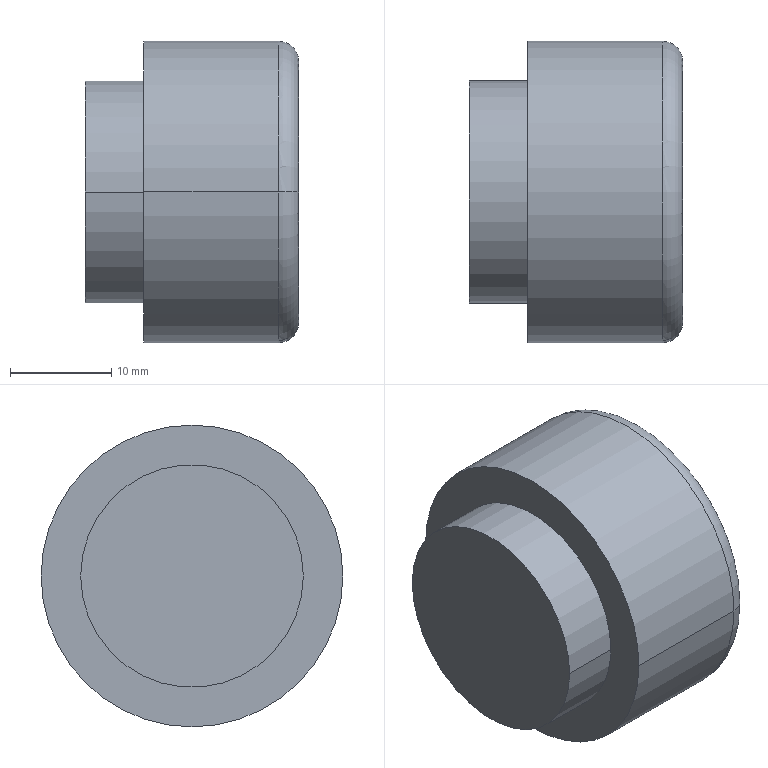Part | STEP file | 7-4-Part3-619-724 | 1 solid | 9 faces | box 21.06 x 29.813 x 29.813 mm | volume 12789 mm3 | cylinder 4 | plane 3 | torus 2 | commonest cylinder face diameters 22 x2 29.813 x2
STEP:
#1=CARTESIAN_POINT('',(0.,0.,0.));
#2=DIRECTION('',(0.,0.,1.));
#3=DIRECTION('',(1.,0.,0.));
#4=AXIS2_PLACEMENT_3D('',#1,#2,#3);
#5=CARTESIAN_POINT('',(19.06,-25.906,0.));
#6=VERTEX_POINT('',#5);
#7=CARTESIAN_POINT('',(19.06,3.906,0.));
#8=VERTEX_POINT('',#7);
#9=CARTESIAN_POINT('',(19.06,-11.,0.));
#10=DIRECTION('',(-1.,0.,0.));
#11=DIRECTION('',(0.,1.,0.));
#12=AXIS2_PLACEMENT_3D('',#9,#10,#11);
#13=CIRCLE('',#12,14.906);
#14=CARTESIAN_POINT('',(19.06,-11.,0.));
#15=DIRECTION('',(1.,0.,0.));
#16=DIRECTION('',(0.,1.,0.));
#17=AXIS2_PLACEMENT_3D('',#14,#15,#16);
#18=TOROIDAL_SURFACE('',#17,12.906,2.);
#19=CARTESIAN_POINT('',(3.142,0.));
#20=CARTESIAN_POINT('',(3.094,0.));
#21=CARTESIAN_POINT('',(2.999,0.));
#22=CARTESIAN_POINT('',(2.856,0.));
#23=CARTESIAN_POINT('',(2.713,0.));
#24=CARTESIAN_POINT('',(2.57,0.));
#25=CARTESIAN_POINT('',(2.428,0.));
#26=CARTESIAN_POINT('',(2.285,0.));
#27=CARTESIAN_POINT('',(2.142,0.));
#28=CARTESIAN_POINT('',(1.999,0.));
#29=CARTESIAN_POINT('',(1.856,0.));
#30=CARTESIAN_POINT('',(1.714,0.));
#31=CARTESIAN_POINT('',(1.571,0.));
#32=CARTESIAN_POINT('',(1.428,0.));
#33=CARTESIAN_POINT('',(1.285,0.));
#34=CARTESIAN_POINT('',(1.142,0.));
#35=CARTESIAN_POINT('',(0.9996,0.));
#36=CARTESIAN_POINT('',(0.8568,0.));
#37=CARTESIAN_POINT('',(0.714,0.));
#38=CARTESIAN_POINT('',(0.5712,0.));
#39=CARTESIAN_POINT('',(0.4284,0.));
#40=CARTESIAN_POINT('',(0.2856,0.));
#41=CARTESIAN_POINT('',(0.1428,0.));
#42=CARTESIAN_POINT('',(0.0476,0.));
#43=CARTESIAN_POINT('',(0.,0.));
#44=B_SPLINE_CURVE_WITH_KNOTS('',3,(#19,#20,#21,#22,#23,#24,#25,#26,#27,#28,#29,#30,#31,#32,#33,#34,#35,#36,#37,#38,#39,#40,#41,#42,#43),.UNSPECIFIED.,.F.,.F.,(4,1,1,1,1,1,1,1,1,1,1,1,1,1,1,1,1,1,1,1,1,1,4),(3.142,3.284,3.427,3.57,3.713,3.856,3.998,4.141,4.284,4.427,4.57,4.712,4.855,4.998,5.141,5.284,5.426,5.569,5.712,5.855,5.998,6.14,6.283),.QUASI_UNIFORM_KNOTS.);
#45=(GEOMETRIC_REPRESENTATION_CONTEXT(2)PARAMETRIC_REPRESENTATION_CONTEXT()REPRESENTATION_CONTEXT('',''));
#46=DEFINITIONAL_REPRESENTATION('',(#44),#45);
#47=PCURVE('',#18,#46);
#48=CARTESIAN_POINT('',(21.06,-11.,0.));
#49=DIRECTION('',(1.,0.,0.));
#50=DIRECTION('',(0.,1.,0.));
#51=AXIS2_PLACEMENT_3D('',#48,#49,#50);
#52=CYLINDRICAL_SURFACE('',#51,14.906);
#53=CARTESIAN_POINT('',(6.283,-2.));
#54=DIRECTION('',(-1.,0.));
#55=VECTOR('',#54,1.);
#56=LINE('',#53,#55);
#57=(GEOMETRIC_REPRESENTATION_CONTEXT(2)PARAMETRIC_REPRESENTATION_CONTEXT()REPRESENTATION_CONTEXT('',''));
#58=DEFINITIONAL_REPRESENTATION('',(#56),#57);
#59=PCURVE('',#52,#58);
#60=SURFACE_CURVE('',#13,(#47,#59),.PCURVE_S1.);
#61=EDGE_CURVE('',#6,#8,#60,.T.);
#62=ORIENTED_EDGE('',*,*,#61,.F.);
#63=CARTESIAN_POINT('',(21.06,-23.906,0.));
#64=VERTEX_POINT('',#63);
#65=CARTESIAN_POINT('',(19.06,-23.906,0.));
#66=DIRECTION('',(0.,0.,1.));
#67=DIRECTION('',(0.,-1.,0.));
#68=AXIS2_PLACEMENT_3D('',#65,#66,#67);
#69=CIRCLE('',#68,2.);
#70=CARTESIAN_POINT('',(3.142,0.));
#71=DIRECTION('',(0.,1.));
#72=VECTOR('',#71,1.);
#73=LINE('',#70,#72);
#74=(GEOMETRIC_REPRESENTATION_CONTEXT(2)PARAMETRIC_REPRESENTATION_CONTEXT()REPRESENTATION_CONTEXT('',''));
#75=DEFINITIONAL_REPRESENTATION('',(#73),#74);
#76=PCURVE('',#18,#75);
#77=CARTESIAN_POINT('',(19.06,-11.,0.));
#78=DIRECTION('',(1.,0.,0.));
#79=DIRECTION('',(0.,1.,0.));
#80=AXIS2_PLACEMENT_3D('',#77,#78,#79);
#81=TOROIDAL_SURFACE('',#80,12.906,2.);
#82=CARTESIAN_POINT('',(3.142,0.));
#83=DIRECTION('',(0.,1.));
#84=VECTOR('',#83,1.);
#85=LINE('',#82,#84);
#86=(GEOMETRIC_REPRESENTATION_CONTEXT(2)PARAMETRIC_REPRESENTATION_CONTEXT()REPRESENTATION_CONTEXT('',''));
#87=DEFINITIONAL_REPRESENTATION('',(#85),#86);
#88=PCURVE('',#81,#87);
#89=SURFACE_CURVE('',#69,(#76,#88),.PCURVE_S1.);
#90=EDGE_CURVE('',#6,#64,#89,.T.);
#91=ORIENTED_EDGE('',*,*,#90,.T.);
#92=CARTESIAN_POINT('',(21.06,1.906,0.));
#93=VERTEX_POINT('',#92);
#94=CARTESIAN_POINT('',(21.06,-11.,0.));
#95=DIRECTION('',(1.,0.,0.));
#96=DIRECTION('',(0.,1.,0.));
#97=AXIS2_PLACEMENT_3D('',#94,#95,#96);
#98=CIRCLE('',#97,12.906);
#99=CARTESIAN_POINT('',(0.,1.571));
#100=DIRECTION('',(1.,0.));
#101=VECTOR('',#100,1.);
#102=LINE('',#99,#101);
#103=(GEOMETRIC_REPRESENTATION_CONTEXT(2)PARAMETRIC_REPRESENTATION_CONTEXT()REPRESENTATION_CONTEXT('',''));
#104=DEFINITIONAL_REPRESENTATION('',(#102),#103);
#105=PCURVE('',#18,#104);
#106=CARTESIAN_POINT('',(21.06,3.906,0.));
#107=DIRECTION('',(1.,0.,0.));
#108=DIRECTION('',(0.,1.,0.));
#109=AXIS2_PLACEMENT_3D('',#106,#107,#108);
#110=PLANE('',#109);
#111=CARTESIAN_POINT('',(-14.906,0.));
#112=DIRECTION('',(1.,0.));
#113=AXIS2_PLACEMENT_2D('',#111,#112);
#114=CIRCLE('',#113,12.906);
#115=(GEOMETRIC_REPRESENTATION_CONTEXT(2)PARAMETRIC_REPRESENTATION_CONTEXT()REPRESENTATION_CONTEXT('',''));
#116=DEFINITIONAL_REPRESENTATION('',(#114),#115);
#117=PCURVE('',#110,#116);
#118=SURFACE_CURVE('',#98,(#105,#117),.PCURVE_S1.);
#119=EDGE_CURVE('',#93,#64,#118,.T.);
#120=ORIENTED_EDGE('',*,*,#119,.F.);
#121=CARTESIAN_POINT('',(19.06,1.906,0.));
#122=DIRECTION('',(0.,0.,-1.));
#123=DIRECTION('',(-1.,0.,0.));
#124=AXIS2_PLACEMENT_3D('',#121,#122,#123);
#125=CIRCLE('',#124,2.);
#126=CARTESIAN_POINT('',(0.,-1.571));
#127=DIRECTION('',(0.,1.));
#128=VECTOR('',#127,1.);
#129=LINE('',#126,#128);
#130=(GEOMETRIC_REPRESENTATION_CONTEXT(2)PARAMETRIC_REPRESENTATION_CONTEXT()REPRESENTATION_CONTEXT('',''));
#131=DEFINITIONAL_REPRESENTATION('',(#129),#130);
#132=PCURVE('',#18,#131);
#133=CARTESIAN_POINT('',(6.283,-1.571));
#134=DIRECTION('',(0.,1.));
#135=VECTOR('',#134,1.);
#136=LINE('',#133,#135);
#137=(GEOMETRIC_REPRESENTATION_CONTEXT(2)PARAMETRIC_REPRESENTATION_CONTEXT()REPRESENTATION_CONTEXT('',''));
#138=DEFINITIONAL_REPRESENTATION('',(#136),#137);
#139=PCURVE('',#81,#138);
#140=SURFACE_CURVE('',#125,(#132,#139),.PCURVE_S1.);
#141=EDGE_CURVE('',#8,#93,#140,.T.);
#142=ORIENTED_EDGE('',*,*,#141,.F.);
#143=EDGE_LOOP('',(#62,#91,#120,#142));
#144=FACE_BOUND('',#143,.T.);
#145=ADVANCED_FACE('',(#144),#18,.T.);
#146=CARTESIAN_POINT('',(5.769,3.906,0.));
#147=VERTEX_POINT('',#146);
#148=CARTESIAN_POINT('',(5.769,-25.906,0.));
#149=VERTEX_POINT('',#148);
#150=CARTESIAN_POINT('',(5.769,-11.,0.));
#151=DIRECTION('',(1.,0.,0.));
#152=DIRECTION('',(0.,1.,0.));
#153=AXIS2_PLACEMENT_3D('',#150,#151,#152);
#154=CIRCLE('',#153,14.906);
#155=CARTESIAN_POINT('',(0.,-15.291));
#156=DIRECTION('',(1.,0.));
#157=VECTOR('',#156,1.);
#158=LINE('',#155,#157);
#159=(GEOMETRIC_REPRESENTATION_CONTEXT(2)PARAMETRIC_REPRESENTATION_CONTEXT()REPRESENTATION_CONTEXT('',''));
#160=DEFINITIONAL_REPRESENTATION('',(#158),#159);
#161=PCURVE('',#52,#160);
#162=CARTESIAN_POINT('',(5.769,0.,0.));
#163=DIRECTION('',(-1.,0.,0.));
#164=DIRECTION('',(0.,-1.,0.));
#165=AXIS2_PLACEMENT_3D('',#162,#163,#164);
#166=PLANE('',#165);
#167=CARTESIAN_POINT('',(-3.906,0.));
#168=CARTESIAN_POINT('',(-3.906,25.819));
#169=CARTESIAN_POINT('',(18.453,12.909));
#170=CARTESIAN_POINT('',(40.813,0.));
#171=CARTESIAN_POINT('',(18.453,-12.909));
#172=CARTESIAN_POINT('',(-3.906,-25.819));
#173=CARTESIAN_POINT('',(-3.906,0.));
#174=(BOUNDED_CURVE()B_SPLINE_CURVE(2,(#167,#168,#169,#170,#171,#172,#173),.UNSPECIFIED.,.T.,.F.)B_SPLINE_CURVE_WITH_KNOTS((1,2,2,2,2,1),(-2.094,0.,2.094,4.189,6.283,8.378),.UNSPECIFIED.)CURVE()GEOMETRIC_REPRESENTATION_ITEM()RATIONAL_B_SPLINE_CURVE((1.,0.5,1.,0.5,1.,0.5,1.))REPRESENTATION_ITEM(''));
#175=(GEOMETRIC_REPRESENTATION_CONTEXT(2)PARAMETRIC_REPRESENTATION_CONTEXT()REPRESENTATION_CONTEXT('',''));
#176=DEFINITIONAL_REPRESENTATION('',(#174),#175);
#177=PCURVE('',#166,#176);
#178=SURFACE_CURVE('',#154,(#161,#177),.PCURVE_S1.);
#179=EDGE_CURVE('',#147,#149,#178,.T.);
#180=ORIENTED_EDGE('',*,*,#179,.T.);
#181=CARTESIAN_POINT('',(21.06,-25.906,0.));
#182=DIRECTION('',(1.,0.,0.));
#183=VECTOR('',#182,1.);
#184=LINE('',#181,#183);
#185=CARTESIAN_POINT('',(3.142,0.));
#186=DIRECTION('',(0.,1.));
#187=VECTOR('',#186,1.);
#188=LINE('',#185,#187);
#189=(GEOMETRIC_REPRESENTATION_CONTEXT(2)PARAMETRIC_REPRESENTATION_CONTEXT()REPRESENTATION_CONTEXT('',''));
#190=DEFINITIONAL_REPRESENTATION('',(#188),#189);
#191=PCURVE('',#52,#190);
#192=CARTESIAN_POINT('',(21.06,-11.,0.));
#193=DIRECTION('',(1.,0.,0.));
#194=DIRECTION('',(0.,1.,0.));
#195=AXIS2_PLACEMENT_3D('',#192,#193,#194);
#196=CYLINDRICAL_SURFACE('',#195,14.906);
#197=CARTESIAN_POINT('',(3.142,0.));
#198=DIRECTION('',(0.,1.));
#199=VECTOR('',#198,1.);
#200=LINE('',#197,#199);
#201=(GEOMETRIC_REPRESENTATION_CONTEXT(2)PARAMETRIC_REPRESENTATION_CONTEXT()REPRESENTATION_CONTEXT('',''));
#202=DEFINITIONAL_REPRESENTATION('',(#200),#201);
#203=PCURVE('',#196,#202);
#204=SURFACE_CURVE('',#184,(#191,#203),.PCURVE_S1.);
#205=EDGE_CURVE('',#149,#6,#204,.T.);
#206=ORIENTED_EDGE('',*,*,#205,.T.);
#207=ORIENTED_EDGE('',*,*,#61,.T.);
#208=CARTESIAN_POINT('',(21.06,3.906,0.));
#209=DIRECTION('',(1.,0.,0.));
#210=VECTOR('',#209,1.);
#211=LINE('',#208,#210);
#212=CARTESIAN_POINT('',(0.,0.));
#213=DIRECTION('',(0.,1.));
#214=VECTOR('',#213,1.);
#215=LINE('',#212,#214);
#216=(GEOMETRIC_REPRESENTATION_CONTEXT(2)PARAMETRIC_REPRESENTATION_CONTEXT()REPRESENTATION_CONTEXT('',''));
#217=DEFINITIONAL_REPRESENTATION('',(#215),#216);
#218=PCURVE('',#52,#217);
#219=CARTESIAN_POINT('',(6.283,0.));
#220=DIRECTION('',(0.,1.));
#221=VECTOR('',#220,1.);
#222=LINE('',#219,#221);
#223=(GEOMETRIC_REPRESENTATION_CONTEXT(2)PARAMETRIC_REPRESENTATION_CONTEXT()REPRESENTATION_CONTEXT('',''));
#224=DEFINITIONAL_REPRESENTATION('',(#222),#223);
#225=PCURVE('',#196,#224);
#226=SURFACE_CURVE('',#211,(#218,#225),.PCURVE_S1.);
#227=EDGE_CURVE('',#147,#8,#226,.T.);
#228=ORIENTED_EDGE('',*,*,#227,.F.);
#229=EDGE_LOOP('',(#180,#206,#207,#228));
#230=FACE_BOUND('',#229,.T.);
#231=ADVANCED_FACE('',(#230),#52,.T.);
#232=CARTESIAN_POINT('',(0.,0.,0.));
#233=VERTEX_POINT('',#232);
#234=CARTESIAN_POINT('',(0.,-22.,0.));
#235=VERTEX_POINT('',#234);
#236=CARTESIAN_POINT('',(0.,-11.,0.));
#237=DIRECTION('',(1.,0.,0.));
#238=DIRECTION('',(0.,1.,0.));
#239=AXIS2_PLACEMENT_3D('',#236,#237,#238);
#240=CIRCLE('',#239,11.);
#241=CARTESIAN_POINT('',(21.06,-11.,0.));
#242=DIRECTION('',(1.,0.,0.));
#243=DIRECTION('',(0.,1.,0.));
#244=AXIS2_PLACEMENT_3D('',#241,#242,#243);
#245=CYLINDRICAL_SURFACE('',#244,11.);
#246=CARTESIAN_POINT('',(0.,-21.06));
#247=DIRECTION('',(1.,0.));
#248=VECTOR('',#247,1.);
#249=LINE('',#246,#248);
#250=(GEOMETRIC_REPRESENTATION_CONTEXT(2)PARAMETRIC_REPRESENTATION_CONTEXT()REPRESENTATION_CONTEXT('',''));
#251=DEFINITIONAL_REPRESENTATION('',(#249),#250);
#252=PCURVE('',#245,#251);
#253=CARTESIAN_POINT('',(0.,-11.,0.));
#254=DIRECTION('',(-1.,0.,0.));
#255=DIRECTION('',(0.,-1.,0.));
#256=AXIS2_PLACEMENT_3D('',#253,#254,#255);
#257=PLANE('',#256);
#258=CARTESIAN_POINT('',(-11.,0.));
#259=CARTESIAN_POINT('',(-11.,19.053));
#260=CARTESIAN_POINT('',(5.5,9.526));
#261=CARTESIAN_POINT('',(22.,0.));
#262=CARTESIAN_POINT('',(5.5,-9.526));
#263=CARTESIAN_POINT('',(-11.,-19.053));
#264=CARTESIAN_POINT('',(-11.,0.));
#265=(BOUNDED_CURVE()B_SPLINE_CURVE(2,(#258,#259,#260,#261,#262,#263,#264),.UNSPECIFIED.,.T.,.F.)B_SPLINE_CURVE_WITH_KNOTS((1,2,2,2,2,1),(-2.094,0.,2.094,4.189,6.283,8.378),.UNSPECIFIED.)CURVE()GEOMETRIC_REPRESENTATION_ITEM()RATIONAL_B_SPLINE_CURVE((1.,0.5,1.,0.5,1.,0.5,1.))REPRESENTATION_ITEM(''));
#266=(GEOMETRIC_REPRESENTATION_CONTEXT(2)PARAMETRIC_REPRESENTATION_CONTEXT()REPRESENTATION_CONTEXT('',''));
#267=DEFINITIONAL_REPRESENTATION('',(#265),#266);
#268=PCURVE('',#257,#267);
#269=SURFACE_CURVE('',#240,(#252,#268),.PCURVE_S1.);
#270=EDGE_CURVE('',#233,#235,#269,.T.);
#271=ORIENTED_EDGE('',*,*,#270,.T.);
#272=CARTESIAN_POINT('',(5.769,-22.,0.));
#273=VERTEX_POINT('',#272);
#274=CARTESIAN_POINT('',(21.06,-22.,0.));
#275=DIRECTION('',(1.,0.,0.));
#276=VECTOR('',#275,1.);
#277=LINE('',#274,#276);
#278=CARTESIAN_POINT('',(3.142,0.));
#279=DIRECTION('',(0.,1.));
#280=VECTOR('',#279,1.);
#281=LINE('',#278,#280);
#282=(GEOMETRIC_REPRESENTATION_CONTEXT(2)PARAMETRIC_REPRESENTATION_CONTEXT()REPRESENTATION_CONTEXT('',''));
#283=DEFINITIONAL_REPRESENTATION('',(#281),#282);
#284=PCURVE('',#245,#283);
#285=CARTESIAN_POINT('',(21.06,-11.,0.));
#286=DIRECTION('',(1.,0.,0.));
#287=DIRECTION('',(0.,1.,0.));
#288=AXIS2_PLACEMENT_3D('',#285,#286,#287);
#289=CYLINDRICAL_SURFACE('',#288,11.);
#290=CARTESIAN_POINT('',(3.142,0.));
#291=DIRECTION('',(0.,1.));
#292=VECTOR('',#291,1.);
#293=LINE('',#290,#292);
#294=(GEOMETRIC_REPRESENTATION_CONTEXT(2)PARAMETRIC_REPRESENTATION_CONTEXT()REPRESENTATION_CONTEXT('',''));
#295=DEFINITIONAL_REPRESENTATION('',(#293),#294);
#296=PCURVE('',#289,#295);
#297=SURFACE_CURVE('',#277,(#284,#296),.PCURVE_S1.);
#298=EDGE_CURVE('',#235,#273,#297,.T.);
#299=ORIENTED_EDGE('',*,*,#298,.T.);
#300=CARTESIAN_POINT('',(5.769,0.,0.));
#301=VERTEX_POINT('',#300);
#302=CARTESIAN_POINT('',(5.769,-11.,0.));
#303=DIRECTION('',(1.,0.,0.));
#304=DIRECTION('',(0.,1.,0.));
#305=AXIS2_PLACEMENT_3D('',#302,#303,#304);
#306=CIRCLE('',#305,11.);
#307=CARTESIAN_POINT('',(0.,-15.291));
#308=DIRECTION('',(1.,0.));
#309=VECTOR('',#308,1.);
#310=LINE('',#307,#309);
#311=(GEOMETRIC_REPRESENTATION_CONTEXT(2)PARAMETRIC_REPRESENTATION_CONTEXT()REPRESENTATION_CONTEXT('',''));
#312=DEFINITIONAL_REPRESENTATION('',(#310),#311);
#313=PCURVE('',#245,#312);
#314=CARTESIAN_POINT('',(0.,0.));
#315=CARTESIAN_POINT('',(0.,19.053));
#316=CARTESIAN_POINT('',(16.5,9.526));
#317=CARTESIAN_POINT('',(33.,0.));
#318=CARTESIAN_POINT('',(16.5,-9.526));
#319=CARTESIAN_POINT('',(0.,-19.053));
#320=CARTESIAN_POINT('',(0.,0.));
#321=(BOUNDED_CURVE()B_SPLINE_CURVE(2,(#314,#315,#316,#317,#318,#319,#320),.UNSPECIFIED.,.T.,.F.)B_SPLINE_CURVE_WITH_KNOTS((1,2,2,2,2,1),(-2.094,0.,2.094,4.189,6.283,8.378),.UNSPECIFIED.)CURVE()GEOMETRIC_REPRESENTATION_ITEM()RATIONAL_B_SPLINE_CURVE((1.,0.5,1.,0.5,1.,0.5,1.))REPRESENTATION_ITEM(''));
#322=(GEOMETRIC_REPRESENTATION_CONTEXT(2)PARAMETRIC_REPRESENTATION_CONTEXT()REPRESENTATION_CONTEXT('',''));
#323=DEFINITIONAL_REPRESENTATION('',(#321),#322);
#324=PCURVE('',#166,#323);
#325=SURFACE_CURVE('',#306,(#313,#324),.PCURVE_S1.);
#326=EDGE_CURVE('',#301,#273,#325,.T.);
#327=ORIENTED_EDGE('',*,*,#326,.F.);
#328=CARTESIAN_POINT('',(21.06,0.,0.));
#329=DIRECTION('',(1.,0.,0.));
#330=VECTOR('',#329,1.);
#331=LINE('',#328,#330);
#332=CARTESIAN_POINT('',(0.,0.));
#333=DIRECTION('',(0.,1.));
#334=VECTOR('',#333,1.);
#335=LINE('',#332,#334);
#336=(GEOMETRIC_REPRESENTATION_CONTEXT(2)PARAMETRIC_REPRESENTATION_CONTEXT()REPRESENTATION_CONTEXT('',''));
#337=DEFINITIONAL_REPRESENTATION('',(#335),#336);
#338=PCURVE('',#245,#337);
#339=CARTESIAN_POINT('',(6.283,0.));
#340=DIRECTION('',(0.,1.));
#341=VECTOR('',#340,1.);
#342=LINE('',#339,#341);
#343=(GEOMETRIC_REPRESENTATION_CONTEXT(2)PARAMETRIC_REPRESENTATION_CONTEXT()REPRESENTATION_CONTEXT('',''));
#344=DEFINITIONAL_REPRESENTATION('',(#342),#343);
#345=PCURVE('',#289,#344);
#346=SURFACE_CURVE('',#331,(#338,#345),.PCURVE_S1.);
#347=EDGE_CURVE('',#233,#301,#346,.T.);
#348=ORIENTED_EDGE('',*,*,#347,.F.);
#349=EDGE_LOOP('',(#271,#299,#327,#348));
#350=FACE_BOUND('',#349,.T.);
#351=ADVANCED_FACE('',(#350),#245,.T.);
#352=ORIENTED_EDGE('',*,*,#270,.F.);
#353=CARTESIAN_POINT('',(0.,-11.,0.));
#354=DIRECTION('',(1.,0.,0.));
#355=DIRECTION('',(0.,1.,0.));
#356=AXIS2_PLACEMENT_3D('',#353,#354,#355);
#357=CIRCLE('',#356,11.);
#358=CARTESIAN_POINT('',(-11.,0.));
#359=CARTESIAN_POINT('',(-11.,19.053));
#360=CARTESIAN_POINT('',(5.5,9.526));
#361=CARTESIAN_POINT('',(22.,0.));
#362=CARTESIAN_POINT('',(5.5,-9.526));
#363=CARTESIAN_POINT('',(-11.,-19.053));
#364=CARTESIAN_POINT('',(-11.,0.));
#365=(BOUNDED_CURVE()B_SPLINE_CURVE(2,(#358,#359,#360,#361,#362,#363,#364),.UNSPECIFIED.,.T.,.F.)B_SPLINE_CURVE_WITH_KNOTS((1,2,2,2,2,1),(-2.094,0.,2.094,4.189,6.283,8.378),.UNSPECIFIED.)CURVE()GEOMETRIC_REPRESENTATION_ITEM()RATIONAL_B_SPLINE_CURVE((1.,0.5,1.,0.5,1.,0.5,1.))REPRESENTATION_ITEM(''));
#366=(GEOMETRIC_REPRESENTATION_CONTEXT(2)PARAMETRIC_REPRESENTATION_CONTEXT()REPRESENTATION_CONTEXT('',''));
#367=DEFINITIONAL_REPRESENTATION('',(#365),#366);
#368=PCURVE('',#257,#367);
#369=CARTESIAN_POINT('',(0.,-21.06));
#370=DIRECTION('',(1.,0.));
#371=VECTOR('',#370,1.);
#372=LINE('',#369,#371);
#373=(GEOMETRIC_REPRESENTATION_CONTEXT(2)PARAMETRIC_REPRESENTATION_CONTEXT()REPRESENTATION_CONTEXT('',''));
#374=DEFINITIONAL_REPRESENTATION('',(#372),#373);
#375=PCURVE('',#289,#374);
#376=SURFACE_CURVE('',#357,(#368,#375),.PCURVE_S1.);
#377=EDGE_CURVE('',#235,#233,#376,.T.);
#378=ORIENTED_EDGE('',*,*,#377,.F.);
#379=EDGE_LOOP('',(#352,#378));
#380=FACE_BOUND('',#379,.T.);
#381=ADVANCED_FACE('',(#380),#257,.T.);
#382=ORIENTED_EDGE('',*,*,#298,.F.);
#383=ORIENTED_EDGE('',*,*,#377,.T.);
#384=ORIENTED_EDGE('',*,*,#347,.T.);
#385=CARTESIAN_POINT('',(5.769,-11.,0.));
#386=DIRECTION('',(1.,0.,0.));
#387=DIRECTION('',(0.,1.,0.));
#388=AXIS2_PLACEMENT_3D('',#385,#386,#387);
#389=CIRCLE('',#388,11.);
#390=CARTESIAN_POINT('',(0.,-15.291));
#391=DIRECTION('',(1.,0.));
#392=VECTOR('',#391,1.);
#393=LINE('',#390,#392);
#394=(GEOMETRIC_REPRESENTATION_CONTEXT(2)PARAMETRIC_REPRESENTATION_CONTEXT()REPRESENTATION_CONTEXT('',''));
#395=DEFINITIONAL_REPRESENTATION('',(#393),#394);
#396=PCURVE('',#289,#395);
#397=CARTESIAN_POINT('',(0.,0.));
#398=CARTESIAN_POINT('',(0.,19.053));
#399=CARTESIAN_POINT('',(16.5,9.526));
#400=CARTESIAN_POINT('',(33.,0.));
#401=CARTESIAN_POINT('',(16.5,-9.526));
#402=CARTESIAN_POINT('',(0.,-19.053));
#403=CARTESIAN_POINT('',(0.,0.));
#404=(BOUNDED_CURVE()B_SPLINE_CURVE(2,(#397,#398,#399,#400,#401,#402,#403),.UNSPECIFIED.,.T.,.F.)B_SPLINE_CURVE_WITH_KNOTS((1,2,2,2,2,1),(-2.094,0.,2.094,4.189,6.283,8.378),.UNSPECIFIED.)CURVE()GEOMETRIC_REPRESENTATION_ITEM()RATIONAL_B_SPLINE_CURVE((1.,0.5,1.,0.5,1.,0.5,1.))REPRESENTATION_ITEM(''));
#405=(GEOMETRIC_REPRESENTATION_CONTEXT(2)PARAMETRIC_REPRESENTATION_CONTEXT()REPRESENTATION_CONTEXT('',''));
#406=DEFINITIONAL_REPRESENTATION('',(#404),#405);
#407=PCURVE('',#166,#406);
#408=SURFACE_CURVE('',#389,(#396,#407),.PCURVE_S1.);
#409=EDGE_CURVE('',#273,#301,#408,.T.);
#410=ORIENTED_EDGE('',*,*,#409,.F.);
#411=EDGE_LOOP('',(#382,#383,#384,#410));
#412=FACE_BOUND('',#411,.T.);
#413=ADVANCED_FACE('',(#412),#289,.T.);
#414=ORIENTED_EDGE('',*,*,#326,.T.);
#415=ORIENTED_EDGE('',*,*,#409,.T.);
#416=EDGE_LOOP('',(#414,#415));
#417=FACE_BOUND('',#416,.T.);
#418=ORIENTED_EDGE('',*,*,#179,.F.);
#419=CARTESIAN_POINT('',(5.769,-11.,0.));
#420=DIRECTION('',(1.,0.,0.));
#421=DIRECTION('',(0.,1.,0.));
#422=AXIS2_PLACEMENT_3D('',#419,#420,#421);
#423=CIRCLE('',#422,14.906);
#424=CARTESIAN_POINT('',(-3.906,0.));
#425=CARTESIAN_POINT('',(-3.906,25.819));
#426=CARTESIAN_POINT('',(18.453,12.909));
#427=CARTESIAN_POINT('',(40.813,0.));
#428=CARTESIAN_POINT('',(18.453,-12.909));
#429=CARTESIAN_POINT('',(-3.906,-25.819));
#430=CARTESIAN_POINT('',(-3.906,0.));
#431=(BOUNDED_CURVE()B_SPLINE_CURVE(2,(#424,#425,#426,#427,#428,#429,#430),.UNSPECIFIED.,.T.,.F.)B_SPLINE_CURVE_WITH_KNOTS((1,2,2,2,2,1),(-2.094,0.,2.094,4.189,6.283,8.378),.UNSPECIFIED.)CURVE()GEOMETRIC_REPRESENTATION_ITEM()RATIONAL_B_SPLINE_CURVE((1.,0.5,1.,0.5,1.,0.5,1.))REPRESENTATION_ITEM(''));
#432=(GEOMETRIC_REPRESENTATION_CONTEXT(2)PARAMETRIC_REPRESENTATION_CONTEXT()REPRESENTATION_CONTEXT('',''));
#433=DEFINITIONAL_REPRESENTATION('',(#431),#432);
#434=PCURVE('',#166,#433);
#435=CARTESIAN_POINT('',(0.,-15.291));
#436=DIRECTION('',(1.,0.));
#437=VECTOR('',#436,1.);
#438=LINE('',#435,#437);
#439=(GEOMETRIC_REPRESENTATION_CONTEXT(2)PARAMETRIC_REPRESENTATION_CONTEXT()REPRESENTATION_CONTEXT('',''));
#440=DEFINITIONAL_REPRESENTATION('',(#438),#439);
#441=PCURVE('',#196,#440);
#442=SURFACE_CURVE('',#423,(#434,#441),.PCURVE_S1.);
#443=EDGE_CURVE('',#149,#147,#442,.T.);
#444=ORIENTED_EDGE('',*,*,#443,.F.);
#445=EDGE_LOOP('',(#418,#444));
#446=FACE_BOUND('',#445,.T.);
#447=ADVANCED_FACE('',(#417,#446),#166,.T.);
#448=ORIENTED_EDGE('',*,*,#205,.F.);
#449=ORIENTED_EDGE('',*,*,#443,.T.);
#450=ORIENTED_EDGE('',*,*,#227,.T.);
#451=CARTESIAN_POINT('',(19.06,-11.,0.));
#452=DIRECTION('',(-1.,0.,0.));
#453=DIRECTION('',(0.,1.,0.));
#454=AXIS2_PLACEMENT_3D('',#451,#452,#453);
#455=CIRCLE('',#454,14.906);
#456=CARTESIAN_POINT('',(6.283,-2.));
#457=DIRECTION('',(-1.,0.));
#458=VECTOR('',#457,1.);
#459=LINE('',#456,#458);
#460=(GEOMETRIC_REPRESENTATION_CONTEXT(2)PARAMETRIC_REPRESENTATION_CONTEXT()REPRESENTATION_CONTEXT('',''));
#461=DEFINITIONAL_REPRESENTATION('',(#459),#460);
#462=PCURVE('',#196,#461);
#463=CARTESIAN_POINT('',(6.283,0.));
#464=DIRECTION('',(-1.,0.));
#465=VECTOR('',#464,1.);
#466=LINE('',#463,#465);
#467=(GEOMETRIC_REPRESENTATION_CONTEXT(2)PARAMETRIC_REPRESENTATION_CONTEXT()REPRESENTATION_CONTEXT('',''));
#468=DEFINITIONAL_REPRESENTATION('',(#466),#467);
#469=PCURVE('',#81,#468);
#470=SURFACE_CURVE('',#455,(#462,#469),.PCURVE_S1.);
#471=EDGE_CURVE('',#8,#6,#470,.T.);
#472=ORIENTED_EDGE('',*,*,#471,.T.);
#473=EDGE_LOOP('',(#448,#449,#450,#472));
#474=FACE_BOUND('',#473,.T.);
#475=ADVANCED_FACE('',(#474),#196,.T.);
#476=ORIENTED_EDGE('',*,*,#119,.T.);
#477=CARTESIAN_POINT('',(21.06,-11.,0.));
#478=DIRECTION('',(1.,0.,0.));
#479=DIRECTION('',(0.,1.,0.));
#480=AXIS2_PLACEMENT_3D('',#477,#478,#479);
#481=CIRCLE('',#480,12.906);
#482=CARTESIAN_POINT('',(-14.906,0.));
#483=DIRECTION('',(1.,0.));
#484=AXIS2_PLACEMENT_2D('',#482,#483);
#485=CIRCLE('',#484,12.906);
#486=(GEOMETRIC_REPRESENTATION_CONTEXT(2)PARAMETRIC_REPRESENTATION_CONTEXT()REPRESENTATION_CONTEXT('',''));
#487=DEFINITIONAL_REPRESENTATION('',(#485),#486);
#488=PCURVE('',#110,#487);
#489=CARTESIAN_POINT('',(0.,1.571));
#490=DIRECTION('',(1.,0.));
#491=VECTOR('',#490,1.);
#492=LINE('',#489,#491);
#493=(GEOMETRIC_REPRESENTATION_CONTEXT(2)PARAMETRIC_REPRESENTATION_CONTEXT()REPRESENTATION_CONTEXT('',''));
#494=DEFINITIONAL_REPRESENTATION('',(#492),#493);
#495=PCURVE('',#81,#494);
#496=SURFACE_CURVE('',#481,(#488,#495),.PCURVE_S1.);
#497=EDGE_CURVE('',#64,#93,#496,.T.);
#498=ORIENTED_EDGE('',*,*,#497,.T.);
#499=EDGE_LOOP('',(#476,#498));
#500=FACE_BOUND('',#499,.T.);
#501=ADVANCED_FACE('',(#500),#110,.T.);
#502=ORIENTED_EDGE('',*,*,#90,.F.);
#503=ORIENTED_EDGE('',*,*,#471,.F.);
#504=ORIENTED_EDGE('',*,*,#141,.T.);
#505=ORIENTED_EDGE('',*,*,#497,.F.);
#506=EDGE_LOOP('',(#502,#503,#504,#505));
#507=FACE_BOUND('',#506,.T.);
#508=ADVANCED_FACE('',(#507),#81,.T.);
#509=CLOSED_SHELL('',(#145,#231,#351,#381,#413,#447,#475,#501,#508));
#510=MANIFOLD_SOLID_BREP('',#509);
#511=(LENGTH_UNIT()NAMED_UNIT(*)SI_UNIT(.MILLI.,.METRE.));
#512=UNCERTAINTY_MEASURE_WITH_UNIT(LENGTH_MEASURE(0.0000001),#511,'','');
#513=(NAMED_UNIT(*)PLANE_ANGLE_UNIT()SI_UNIT($,.RADIAN.));
#514=(NAMED_UNIT(*)SI_UNIT($,.STERADIAN.)SOLID_ANGLE_UNIT());
#515=(GEOMETRIC_REPRESENTATION_CONTEXT(3)GLOBAL_UNCERTAINTY_ASSIGNED_CONTEXT((#512))GLOBAL_UNIT_ASSIGNED_CONTEXT((#511,#513,#514))REPRESENTATION_CONTEXT('',''));
#516=ADVANCED_BREP_SHAPE_REPRESENTATION('',(#4,#510),#515);